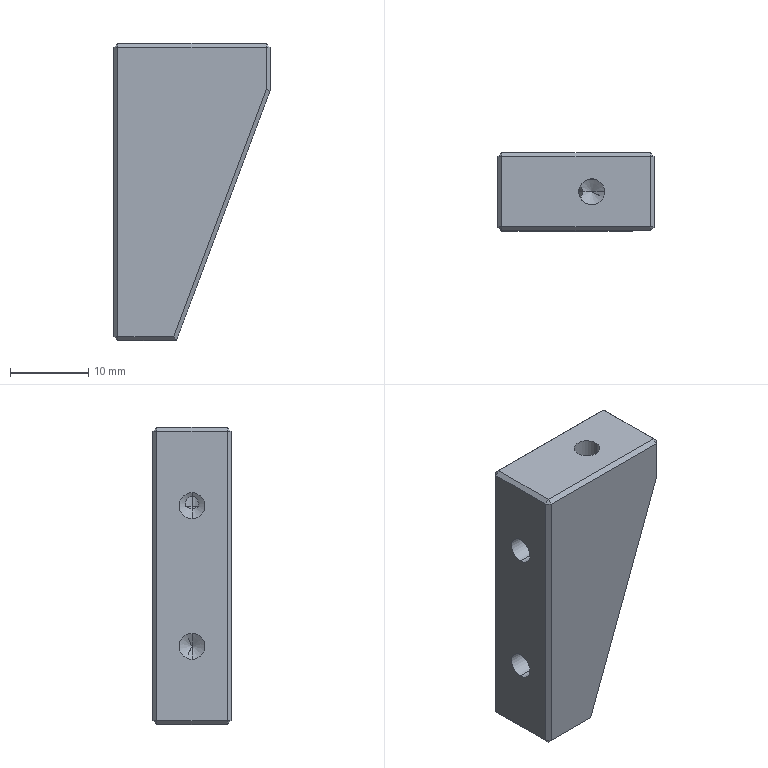Part | STEP file | ND25021-01-JDKM-59-TL | 1 solid | 38 faces | box 20 x 10 x 38 mm | volume 5383 mm3 | plane 26 | cylinder 6 | cone 6 | commonest cylinder face diameters 3.3 x6